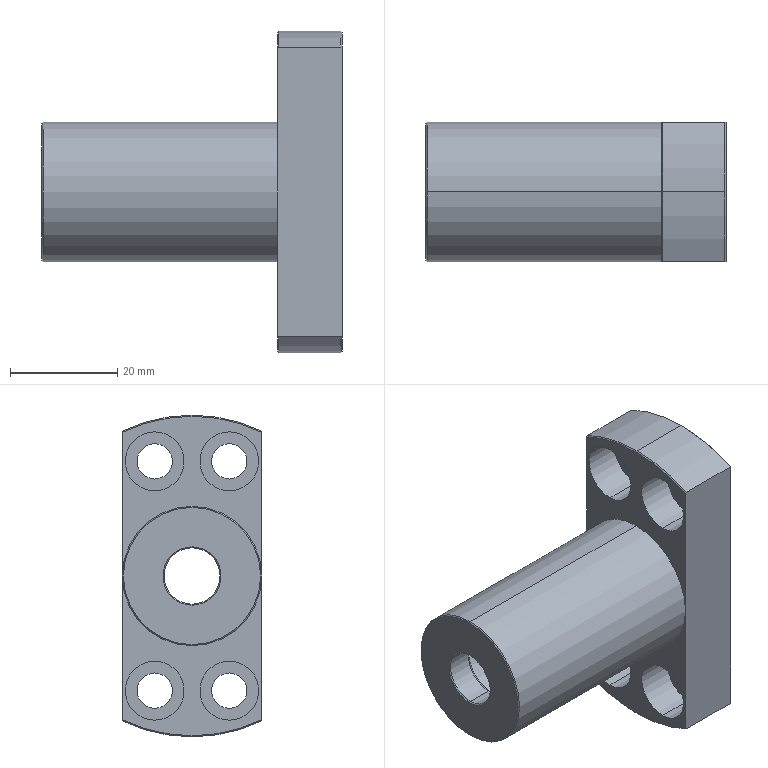Part | SolidWorks | features Chamfer 3, ICE 2, 3DProfileFeature 1, HoleWzd 1, Revolution 1 | 1 solid | 50 faces | box 56 x 26 x 60 mm | volume 18631 mm3 | cylinder 25 | cone 14 | plane 11 | commonest cylinder face diameters 6.6 x8 11 x8 60 x3 10.5 x2 22 x2 26 x2
STEP:
#1=CARTESIAN_POINT('',(5.,0.,5.25));
#2=VERTEX_POINT('',#1);
#3=CARTESIAN_POINT('',(5.,0.,-5.25));
#4=VERTEX_POINT('',#3);
#5=CARTESIAN_POINT('',(5.,0.,0.));
#6=DIRECTION('',(1.,0.,0.));
#7=DIRECTION('',(0.,0.,1.));
#8=AXIS2_PLACEMENT_3D('',#5,#6,#7);
#9=CIRCLE('',#8,5.25);
#10=EDGE_CURVE('',#2,#4,#9,.T.);
#11=ORIENTED_EDGE('',*,*,#10,.F.);
#12=CARTESIAN_POINT('',(6.,0.,6.25));
#13=VERTEX_POINT('',#12);
#14=CARTESIAN_POINT('',(6.,0.,6.25));
#15=DIRECTION('',(0.7071,0.,0.7071));
#16=VECTOR('',#15,1000.);
#17=LINE('',#14,#16);
#18=EDGE_CURVE('',#2,#13,#17,.T.);
#19=ORIENTED_EDGE('',*,*,#18,.T.);
#20=CARTESIAN_POINT('',(6.,0.,-6.25));
#21=VERTEX_POINT('',#20);
#22=CARTESIAN_POINT('',(6.,0.,0.));
#23=DIRECTION('',(-1.,0.,0.));
#24=DIRECTION('',(0.,0.,1.));
#25=AXIS2_PLACEMENT_3D('',#22,#23,#24);
#26=CIRCLE('',#25,6.25);
#27=EDGE_CURVE('',#21,#13,#26,.T.);
#28=ORIENTED_EDGE('',*,*,#27,.F.);
#29=CARTESIAN_POINT('',(6.,0.,-6.25));
#30=DIRECTION('',(0.7071,0.,-0.7071));
#31=VECTOR('',#30,1000.);
#32=LINE('',#29,#31);
#33=EDGE_CURVE('',#4,#21,#32,.T.);
#34=ORIENTED_EDGE('',*,*,#33,.F.);
#35=EDGE_LOOP('',(#11,#19,#28,#34));
#36=FACE_OUTER_BOUND('',#35,.T.);
#37=CARTESIAN_POINT('',(6.,0.,0.));
#38=DIRECTION('',(1.,0.,0.));
#39=DIRECTION('',(0.,0.,-1.));
#40=AXIS2_PLACEMENT_3D('',#37,#38,#39);
#41=CONICAL_SURFACE('',#40,6.25,0.7854);
#42=ADVANCED_FACE('',(#36),#41,.F.);
#43=CARTESIAN_POINT('',(55.8,0.,11.));
#44=VERTEX_POINT('',#43);
#45=CARTESIAN_POINT('',(55.8,0.,-11.));
#46=VERTEX_POINT('',#45);
#47=CARTESIAN_POINT('',(55.8,0.,0.));
#48=DIRECTION('',(1.,0.,0.));
#49=DIRECTION('',(0.,0.,1.));
#50=AXIS2_PLACEMENT_3D('',#47,#48,#49);
#51=CIRCLE('',#50,11.);
#52=EDGE_CURVE('',#44,#46,#51,.T.);
#53=ORIENTED_EDGE('',*,*,#52,.F.);
#54=CARTESIAN_POINT('',(56.,0.,11.2));
#55=VERTEX_POINT('',#54);
#56=CARTESIAN_POINT('',(56.,0.,11.2));
#57=DIRECTION('',(0.7071,0.,0.7071));
#58=VECTOR('',#57,1000.);
#59=LINE('',#56,#58);
#60=EDGE_CURVE('',#44,#55,#59,.T.);
#61=ORIENTED_EDGE('',*,*,#60,.T.);
#62=CARTESIAN_POINT('',(56.,0.,-11.2));
#63=VERTEX_POINT('',#62);
#64=CARTESIAN_POINT('',(56.,0.,0.));
#65=DIRECTION('',(-1.,0.,0.));
#66=DIRECTION('',(0.,0.,1.));
#67=AXIS2_PLACEMENT_3D('',#64,#65,#66);
#68=CIRCLE('',#67,11.2);
#69=EDGE_CURVE('',#63,#55,#68,.T.);
#70=ORIENTED_EDGE('',*,*,#69,.F.);
#71=CARTESIAN_POINT('',(56.,0.,-11.2));
#72=DIRECTION('',(0.7071,0.,-0.7071));
#73=VECTOR('',#72,1000.);
#74=LINE('',#71,#73);
#75=EDGE_CURVE('',#46,#63,#74,.T.);
#76=ORIENTED_EDGE('',*,*,#75,.F.);
#77=EDGE_LOOP('',(#53,#61,#70,#76));
#78=FACE_OUTER_BOUND('',#77,.T.);
#79=CARTESIAN_POINT('',(56.,0.,0.));
#80=DIRECTION('',(1.,0.,0.));
#81=DIRECTION('',(0.,0.,-1.));
#82=AXIS2_PLACEMENT_3D('',#79,#80,#81);
#83=CONICAL_SURFACE('',#82,11.2,0.7854);
#84=ADVANCED_FACE('',(#78),#83,.F.);
#85=CARTESIAN_POINT('',(0.,0.,12.8));
#86=VERTEX_POINT('',#85);
#87=CARTESIAN_POINT('',(0.,0.,-12.8));
#88=VERTEX_POINT('',#87);
#89=CARTESIAN_POINT('',(0.,0.,0.));
#90=DIRECTION('',(-1.,0.,0.));
#91=DIRECTION('',(0.,0.,-1.));
#92=AXIS2_PLACEMENT_3D('',#89,#90,#91);
#93=CIRCLE('',#92,12.8);
#94=EDGE_CURVE('',#86,#88,#93,.T.);
#95=ORIENTED_EDGE('',*,*,#94,.F.);
#96=CARTESIAN_POINT('',(0.2,0.,13.));
#97=VERTEX_POINT('',#96);
#98=CARTESIAN_POINT('',(0.,0.,12.8));
#99=DIRECTION('',(0.7071,0.,0.7071));
#100=VECTOR('',#99,1000.);
#101=LINE('',#98,#100);
#102=EDGE_CURVE('',#86,#97,#101,.T.);
#103=ORIENTED_EDGE('',*,*,#102,.T.);
#104=CARTESIAN_POINT('',(0.2,0.,-13.));
#105=VERTEX_POINT('',#104);
#106=CARTESIAN_POINT('',(0.2,0.,0.));
#107=DIRECTION('',(1.,0.,0.));
#108=DIRECTION('',(0.,0.,-1.));
#109=AXIS2_PLACEMENT_3D('',#106,#107,#108);
#110=CIRCLE('',#109,13.);
#111=EDGE_CURVE('',#105,#97,#110,.T.);
#112=ORIENTED_EDGE('',*,*,#111,.F.);
#113=CARTESIAN_POINT('',(0.,0.,-12.8));
#114=DIRECTION('',(0.7071,0.,-0.7071));
#115=VECTOR('',#114,1000.);
#116=LINE('',#113,#115);
#117=EDGE_CURVE('',#88,#105,#116,.T.);
#118=ORIENTED_EDGE('',*,*,#117,.F.);
#119=EDGE_LOOP('',(#95,#103,#112,#118));
#120=FACE_OUTER_BOUND('',#119,.T.);
#121=CARTESIAN_POINT('',(0.,0.,0.));
#122=DIRECTION('',(1.,0.,0.));
#123=DIRECTION('',(0.,0.,-1.));
#124=AXIS2_PLACEMENT_3D('',#121,#122,#123);
#125=CONICAL_SURFACE('',#124,12.8,0.7854);
#126=ADVANCED_FACE('',(#120),#125,.T.);
#127=CARTESIAN_POINT('',(0.2,0.,-5.25));
#128=VERTEX_POINT('',#127);
#129=CARTESIAN_POINT('',(0.2,0.,5.25));
#130=VERTEX_POINT('',#129);
#131=CARTESIAN_POINT('',(0.2,0.,0.));
#132=DIRECTION('',(-1.,0.,0.));
#133=DIRECTION('',(0.,0.,-1.));
#134=AXIS2_PLACEMENT_3D('',#131,#132,#133);
#135=CIRCLE('',#134,5.25);
#136=EDGE_CURVE('',#128,#130,#135,.T.);
#137=ORIENTED_EDGE('',*,*,#136,.F.);
#138=CARTESIAN_POINT('',(0.,0.,-5.45));
#139=VERTEX_POINT('',#138);
#140=CARTESIAN_POINT('',(0.2,0.,-5.25));
#141=DIRECTION('',(-0.7071,0.,-0.7071));
#142=VECTOR('',#141,1000.);
#143=LINE('',#140,#142);
#144=EDGE_CURVE('',#128,#139,#143,.T.);
#145=ORIENTED_EDGE('',*,*,#144,.T.);
#146=CARTESIAN_POINT('',(0.,0.,5.45));
#147=VERTEX_POINT('',#146);
#148=CARTESIAN_POINT('',(0.,0.,0.));
#149=DIRECTION('',(1.,0.,0.));
#150=DIRECTION('',(0.,0.,-1.));
#151=AXIS2_PLACEMENT_3D('',#148,#149,#150);
#152=CIRCLE('',#151,5.45);
#153=EDGE_CURVE('',#147,#139,#152,.T.);
#154=ORIENTED_EDGE('',*,*,#153,.F.);
#155=CARTESIAN_POINT('',(0.2,0.,5.25));
#156=DIRECTION('',(-0.7071,0.,0.7071));
#157=VECTOR('',#156,1000.);
#158=LINE('',#155,#157);
#159=EDGE_CURVE('',#130,#147,#158,.T.);
#160=ORIENTED_EDGE('',*,*,#159,.F.);
#161=EDGE_LOOP('',(#137,#145,#154,#160));
#162=FACE_OUTER_BOUND('',#161,.T.);
#163=CARTESIAN_POINT('',(0.2,0.,0.));
#164=DIRECTION('',(-1.,0.,0.));
#165=DIRECTION('',(0.,0.,1.));
#166=AXIS2_PLACEMENT_3D('',#163,#164,#165);
#167=CONICAL_SURFACE('',#166,5.25,0.7854);
#168=ADVANCED_FACE('',(#162),#167,.F.);
#169=CARTESIAN_POINT('',(56.,0.,29.8));
#170=VERTEX_POINT('',#169);
#171=CARTESIAN_POINT('',(56.,-13.,26.815));
#172=VERTEX_POINT('',#171);
#173=CARTESIAN_POINT('',(56.,0.,0.));
#174=DIRECTION('',(1.,0.,0.));
#175=DIRECTION('',(0.,0.,1.));
#176=AXIS2_PLACEMENT_3D('',#173,#174,#175);
#177=CIRCLE('',#176,29.8);
#178=EDGE_CURVE('',#170,#172,#177,.T.);
#179=ORIENTED_EDGE('',*,*,#178,.F.);
#180=CARTESIAN_POINT('',(55.8,0.,30.));
#181=VERTEX_POINT('',#180);
#182=CARTESIAN_POINT('',(55.8,0.,30.));
#183=DIRECTION('',(-0.7071,0.,0.7071));
#184=VECTOR('',#183,1000.);
#185=LINE('',#182,#184);
#186=EDGE_CURVE('',#170,#181,#185,.T.);
#187=ORIENTED_EDGE('',*,*,#186,.T.);
#188=CARTESIAN_POINT('',(55.8,-13.,27.037));
#189=VERTEX_POINT('',#188);
#190=CARTESIAN_POINT('',(55.8,0.,0.));
#191=DIRECTION('',(-1.,0.,0.));
#192=DIRECTION('',(0.,0.,1.));
#193=AXIS2_PLACEMENT_3D('',#190,#191,#192);
#194=CIRCLE('',#193,30.);
#195=EDGE_CURVE('',#189,#181,#194,.T.);
#196=ORIENTED_EDGE('',*,*,#195,.F.);
#197=CARTESIAN_POINT('',(56.,-13.,26.815));
#198=CARTESIAN_POINT('',(55.933,-13.,26.889));
#199=CARTESIAN_POINT('',(55.867,-13.,26.963));
#200=CARTESIAN_POINT('',(55.8,-13.,27.037));
#201=B_SPLINE_CURVE_WITH_KNOTS('',3,(#197,#198,#199,#200),.UNSPECIFIED.,.F.,.F.,(4,4),(0.,0.0002989),.UNSPECIFIED.);
#202=EDGE_CURVE('',#172,#189,#201,.T.);
#203=ORIENTED_EDGE('',*,*,#202,.F.);
#204=EDGE_LOOP('',(#179,#187,#196,#203));
#205=FACE_OUTER_BOUND('',#204,.T.);
#206=CARTESIAN_POINT('',(55.8,0.,0.));
#207=DIRECTION('',(-1.,0.,0.));
#208=DIRECTION('',(0.,0.,1.));
#209=AXIS2_PLACEMENT_3D('',#206,#207,#208);
#210=CONICAL_SURFACE('',#209,30.,0.7854);
#211=ADVANCED_FACE('',(#205),#210,.T.);
#212=CARTESIAN_POINT('',(44.,0.,-29.8));
#213=VERTEX_POINT('',#212);
#214=CARTESIAN_POINT('',(44.,-13.,-26.815));
#215=VERTEX_POINT('',#214);
#216=CARTESIAN_POINT('',(44.,0.,0.));
#217=DIRECTION('',(-1.,0.,0.));
#218=DIRECTION('',(0.,0.,-1.));
#219=AXIS2_PLACEMENT_3D('',#216,#217,#218);
#220=CIRCLE('',#219,29.8);
#221=EDGE_CURVE('',#213,#215,#220,.T.);
#222=ORIENTED_EDGE('',*,*,#221,.F.);
#223=CARTESIAN_POINT('',(44.2,0.,-30.));
#224=VERTEX_POINT('',#223);
#225=CARTESIAN_POINT('',(44.,0.,-29.8));
#226=DIRECTION('',(0.7071,0.,-0.7071));
#227=VECTOR('',#226,1000.);
#228=LINE('',#225,#227);
#229=EDGE_CURVE('',#213,#224,#228,.T.);
#230=ORIENTED_EDGE('',*,*,#229,.T.);
#231=CARTESIAN_POINT('',(44.2,-13.,-27.037));
#232=VERTEX_POINT('',#231);
#233=CARTESIAN_POINT('',(44.2,0.,0.));
#234=DIRECTION('',(1.,0.,0.));
#235=DIRECTION('',(0.,0.,-1.));
#236=AXIS2_PLACEMENT_3D('',#233,#234,#235);
#237=CIRCLE('',#236,30.);
#238=EDGE_CURVE('',#232,#224,#237,.T.);
#239=ORIENTED_EDGE('',*,*,#238,.F.);
#240=CARTESIAN_POINT('',(44.,-13.,-26.815));
#241=CARTESIAN_POINT('',(44.067,-13.,-26.889));
#242=CARTESIAN_POINT('',(44.133,-13.,-26.963));
#243=CARTESIAN_POINT('',(44.2,-13.,-27.037));
#244=B_SPLINE_CURVE_WITH_KNOTS('',3,(#240,#241,#242,#243),.UNSPECIFIED.,.F.,.F.,(4,4),(0.,0.0002989),.UNSPECIFIED.);
#245=EDGE_CURVE('',#215,#232,#244,.T.);
#246=ORIENTED_EDGE('',*,*,#245,.F.);
#247=EDGE_LOOP('',(#222,#230,#239,#246));
#248=FACE_OUTER_BOUND('',#247,.T.);
#249=CARTESIAN_POINT('',(44.,0.,0.));
#250=DIRECTION('',(1.,0.,0.));
#251=DIRECTION('',(0.,0.,-1.));
#252=AXIS2_PLACEMENT_3D('',#249,#250,#251);
#253=CONICAL_SURFACE('',#252,29.8,0.7854);
#254=ADVANCED_FACE('',(#248),#253,.T.);
#255=CARTESIAN_POINT('',(50.8,-6.953,15.899));
#256=VERTEX_POINT('',#255);
#257=CARTESIAN_POINT('',(50.8,-6.953,26.899));
#258=VERTEX_POINT('',#257);
#259=CARTESIAN_POINT('',(50.8,-6.953,21.399));
#260=DIRECTION('',(-1.,0.,0.));
#261=DIRECTION('',(0.,0.,1.));
#262=AXIS2_PLACEMENT_3D('',#259,#260,#261);
#263=CIRCLE('',#262,5.5);
#264=EDGE_CURVE('',#256,#258,#263,.T.);
#265=ORIENTED_EDGE('',*,*,#264,.F.);
#266=CARTESIAN_POINT('',(44.,-6.953,15.899));
#267=VERTEX_POINT('',#266);
#268=CARTESIAN_POINT('',(44.,-6.953,15.899));
#269=DIRECTION('',(-1.,0.,0.));
#270=VECTOR('',#269,1000.);
#271=LINE('',#268,#270);
#272=EDGE_CURVE('',#256,#267,#271,.T.);
#273=ORIENTED_EDGE('',*,*,#272,.T.);
#274=CARTESIAN_POINT('',(44.,-6.953,26.899));
#275=VERTEX_POINT('',#274);
#276=CARTESIAN_POINT('',(44.,-6.953,21.399));
#277=DIRECTION('',(-1.,0.,0.));
#278=DIRECTION('',(0.,0.,1.));
#279=AXIS2_PLACEMENT_3D('',#276,#277,#278);
#280=CIRCLE('',#279,5.5);
#281=EDGE_CURVE('',#267,#275,#280,.T.);
#282=ORIENTED_EDGE('',*,*,#281,.T.);
#283=CARTESIAN_POINT('',(44.,-6.953,26.899));
#284=DIRECTION('',(-1.,0.,0.));
#285=VECTOR('',#284,1000.);
#286=LINE('',#283,#285);
#287=EDGE_CURVE('',#258,#275,#286,.T.);
#288=ORIENTED_EDGE('',*,*,#287,.F.);
#289=EDGE_LOOP('',(#265,#273,#282,#288));
#290=FACE_OUTER_BOUND('',#289,.T.);
#291=CARTESIAN_POINT('',(44.,-6.953,21.399));
#292=DIRECTION('',(-1.,0.,0.));
#293=DIRECTION('',(0.,0.,1.));
#294=AXIS2_PLACEMENT_3D('',#291,#292,#293);
#295=CYLINDRICAL_SURFACE('',#294,5.5);
#296=ADVANCED_FACE('',(#290),#295,.F.);
#297=CARTESIAN_POINT('',(56.,-6.953,18.099));
#298=VERTEX_POINT('',#297);
#299=CARTESIAN_POINT('',(56.,-6.953,24.699));
#300=VERTEX_POINT('',#299);
#301=CARTESIAN_POINT('',(56.,-6.953,21.399));
#302=DIRECTION('',(-1.,0.,0.));
#303=DIRECTION('',(0.,0.,1.));
#304=AXIS2_PLACEMENT_3D('',#301,#302,#303);
#305=CIRCLE('',#304,3.3);
#306=EDGE_CURVE('',#298,#300,#305,.T.);
#307=ORIENTED_EDGE('',*,*,#306,.F.);
#308=CARTESIAN_POINT('',(50.8,-6.953,18.099));
#309=VERTEX_POINT('',#308);
#310=CARTESIAN_POINT('',(44.,-6.953,18.099));
#311=DIRECTION('',(-1.,0.,0.));
#312=VECTOR('',#311,1000.);
#313=LINE('',#310,#312);
#314=EDGE_CURVE('',#298,#309,#313,.T.);
#315=ORIENTED_EDGE('',*,*,#314,.T.);
#316=CARTESIAN_POINT('',(50.8,-6.953,24.699));
#317=VERTEX_POINT('',#316);
#318=CARTESIAN_POINT('',(50.8,-6.953,21.399));
#319=DIRECTION('',(-1.,0.,0.));
#320=DIRECTION('',(0.,0.,1.));
#321=AXIS2_PLACEMENT_3D('',#318,#319,#320);
#322=CIRCLE('',#321,3.3);
#323=EDGE_CURVE('',#309,#317,#322,.T.);
#324=ORIENTED_EDGE('',*,*,#323,.T.);
#325=CARTESIAN_POINT('',(44.,-6.953,24.699));
#326=DIRECTION('',(-1.,0.,0.));
#327=VECTOR('',#326,1000.);
#328=LINE('',#325,#327);
#329=EDGE_CURVE('',#300,#317,#328,.T.);
#330=ORIENTED_EDGE('',*,*,#329,.F.);
#331=EDGE_LOOP('',(#307,#315,#324,#330));
#332=FACE_OUTER_BOUND('',#331,.T.);
#333=CARTESIAN_POINT('',(44.,-6.953,21.399));
#334=DIRECTION('',(-1.,0.,0.));
#335=DIRECTION('',(0.,0.,1.));
#336=AXIS2_PLACEMENT_3D('',#333,#334,#335);
#337=CYLINDRICAL_SURFACE('',#336,3.3);
#338=ADVANCED_FACE('',(#332),#337,.F.);
#339=CARTESIAN_POINT('',(50.8,6.953,15.899));
#340=VERTEX_POINT('',#339);
#341=CARTESIAN_POINT('',(50.8,6.953,26.899));
#342=VERTEX_POINT('',#341);
#343=CARTESIAN_POINT('',(50.8,6.953,21.399));
#344=DIRECTION('',(-1.,0.,0.));
#345=DIRECTION('',(0.,0.,1.));
#346=AXIS2_PLACEMENT_3D('',#343,#344,#345);
#347=CIRCLE('',#346,5.5);
#348=EDGE_CURVE('',#340,#342,#347,.T.);
#349=ORIENTED_EDGE('',*,*,#348,.F.);
#350=CARTESIAN_POINT('',(44.,6.953,15.899));
#351=VERTEX_POINT('',#350);
#352=CARTESIAN_POINT('',(44.,6.953,15.899));
#353=DIRECTION('',(-1.,0.,0.));
#354=VECTOR('',#353,1000.);
#355=LINE('',#352,#354);
#356=EDGE_CURVE('',#340,#351,#355,.T.);
#357=ORIENTED_EDGE('',*,*,#356,.T.);
#358=CARTESIAN_POINT('',(44.,6.953,26.899));
#359=VERTEX_POINT('',#358);
#360=CARTESIAN_POINT('',(44.,6.953,21.399));
#361=DIRECTION('',(-1.,0.,0.));
#362=DIRECTION('',(0.,0.,1.));
#363=AXIS2_PLACEMENT_3D('',#360,#361,#362);
#364=CIRCLE('',#363,5.5);
#365=EDGE_CURVE('',#351,#359,#364,.T.);
#366=ORIENTED_EDGE('',*,*,#365,.T.);
#367=CARTESIAN_POINT('',(44.,6.953,26.899));
#368=DIRECTION('',(-1.,0.,0.));
#369=VECTOR('',#368,1000.);
#370=LINE('',#367,#369);
#371=EDGE_CURVE('',#342,#359,#370,.T.);
#372=ORIENTED_EDGE('',*,*,#371,.F.);
#373=EDGE_LOOP('',(#349,#357,#366,#372));
#374=FACE_OUTER_BOUND('',#373,.T.);
#375=CARTESIAN_POINT('',(44.,6.953,21.399));
#376=DIRECTION('',(-1.,0.,0.));
#377=DIRECTION('',(0.,0.,1.));
#378=AXIS2_PLACEMENT_3D('',#375,#376,#377);
#379=CYLINDRICAL_SURFACE('',#378,5.5);
#380=ADVANCED_FACE('',(#374),#379,.F.);
#381=CARTESIAN_POINT('',(56.,6.953,18.099));
#382=VERTEX_POINT('',#381);
#383=CARTESIAN_POINT('',(56.,6.953,24.699));
#384=VERTEX_POINT('',#383);
#385=CARTESIAN_POINT('',(56.,6.953,21.399));
#386=DIRECTION('',(-1.,0.,0.));
#387=DIRECTION('',(0.,0.,1.));
#388=AXIS2_PLACEMENT_3D('',#385,#386,#387);
#389=CIRCLE('',#388,3.3);
#390=EDGE_CURVE('',#382,#384,#389,.T.);
#391=ORIENTED_EDGE('',*,*,#390,.F.);
#392=CARTESIAN_POINT('',(50.8,6.953,18.099));
#393=VERTEX_POINT('',#392);
#394=CARTESIAN_POINT('',(44.,6.953,18.099));
#395=DIRECTION('',(-1.,0.,0.));
#396=VECTOR('',#395,1000.);
#397=LINE('',#394,#396);
#398=EDGE_CURVE('',#382,#393,#397,.T.);
#399=ORIENTED_EDGE('',*,*,#398,.T.);
#400=CARTESIAN_POINT('',(50.8,6.953,24.699));
#401=VERTEX_POINT('',#400);
#402=CARTESIAN_POINT('',(50.8,6.953,21.399));
#403=DIRECTION('',(-1.,0.,0.));
#404=DIRECTION('',(0.,0.,1.));
#405=AXIS2_PLACEMENT_3D('',#402,#403,#404);
#406=CIRCLE('',#405,3.3);
#407=EDGE_CURVE('',#393,#401,#406,.T.);
#408=ORIENTED_EDGE('',*,*,#407,.T.);
#409=CARTESIAN_POINT('',(44.,6.953,24.699));
#410=DIRECTION('',(-1.,0.,0.));
#411=VECTOR('',#410,1000.);
#412=LINE('',#409,#411);
#413=EDGE_CURVE('',#384,#401,#412,.T.);
#414=ORIENTED_EDGE('',*,*,#413,.F.);
#415=EDGE_LOOP('',(#391,#399,#408,#414));
#416=FACE_OUTER_BOUND('',#415,.T.);
#417=CARTESIAN_POINT('',(44.,6.953,21.399));
#418=DIRECTION('',(-1.,0.,0.));
#419=DIRECTION('',(0.,0.,1.));
#420=AXIS2_PLACEMENT_3D('',#417,#418,#419);
#421=CYLINDRICAL_SURFACE('',#420,3.3);
#422=ADVANCED_FACE('',(#416),#421,.F.);
#423=CARTESIAN_POINT('',(50.8,6.953,-26.899));
#424=VERTEX_POINT('',#423);
#425=CARTESIAN_POINT('',(50.8,6.953,-15.899));
#426=VERTEX_POINT('',#425);
#427=CARTESIAN_POINT('',(50.8,6.953,-21.399));
#428=DIRECTION('',(-1.,0.,0.));
#429=DIRECTION('',(0.,0.,1.));
#430=AXIS2_PLACEMENT_3D('',#427,#428,#429);
#431=CIRCLE('',#430,5.5);
#432=EDGE_CURVE('',#424,#426,#431,.T.);
#433=ORIENTED_EDGE('',*,*,#432,.F.);
#434=CARTESIAN_POINT('',(44.,6.953,-26.899));
#435=VERTEX_POINT('',#434);
#436=CARTESIAN_POINT('',(44.,6.953,-26.899));
#437=DIRECTION('',(-1.,0.,0.));
#438=VECTOR('',#437,1000.);
#439=LINE('',#436,#438);
#440=EDGE_CURVE('',#424,#435,#439,.T.);
#441=ORIENTED_EDGE('',*,*,#440,.T.);
#442=CARTESIAN_POINT('',(44.,6.953,-15.899));
#443=VERTEX_POINT('',#442);
#444=CARTESIAN_POINT('',(44.,6.953,-21.399));
#445=DIRECTION('',(-1.,0.,0.));
#446=DIRECTION('',(0.,0.,1.));
#447=AXIS2_PLACEMENT_3D('',#444,#445,#446);
#448=CIRCLE('',#447,5.5);
#449=EDGE_CURVE('',#435,#443,#448,.T.);
#450=ORIENTED_EDGE('',*,*,#449,.T.);
#451=CARTESIAN_POINT('',(44.,6.953,-15.899));
#452=DIRECTION('',(-1.,0.,0.));
#453=VECTOR('',#452,1000.);
#454=LINE('',#451,#453);
#455=EDGE_CURVE('',#426,#443,#454,.T.);
#456=ORIENTED_EDGE('',*,*,#455,.F.);
#457=EDGE_LOOP('',(#433,#441,#450,#456));
#458=FACE_OUTER_BOUND('',#457,.T.);
#459=CARTESIAN_POINT('',(44.,6.953,-21.399));
#460=DIRECTION('',(-1.,0.,0.));
#461=DIRECTION('',(0.,0.,1.));
#462=AXIS2_PLACEMENT_3D('',#459,#460,#461);
#463=CYLINDRICAL_SURFACE('',#462,5.5);
#464=ADVANCED_FACE('',(#458),#463,.F.);
#465=CARTESIAN_POINT('',(56.,6.953,-24.699));
#466=VERTEX_POINT('',#465);
#467=CARTESIAN_POINT('',(56.,6.953,-18.099));
#468=VERTEX_POINT('',#467);
#469=CARTESIAN_POINT('',(56.,6.953,-21.399));
#470=DIRECTION('',(-1.,0.,0.));
#471=DIRECTION('',(0.,0.,1.));
#472=AXIS2_PLACEMENT_3D('',#469,#470,#471);
#473=CIRCLE('',#472,3.3);
#474=EDGE_CURVE('',#466,#468,#473,.T.);
#475=ORIENTED_EDGE('',*,*,#474,.F.);
#476=CARTESIAN_POINT('',(50.8,6.953,-24.699));
#477=VERTEX_POINT('',#476);
#478=CARTESIAN_POINT('',(44.,6.953,-24.699));
#479=DIRECTION('',(-1.,0.,0.));
#480=VECTOR('',#479,1000.);
#481=LINE('',#478,#480);
#482=EDGE_CURVE('',#466,#477,#481,.T.);
#483=ORIENTED_EDGE('',*,*,#482,.T.);
#484=CARTESIAN_POINT('',(50.8,6.953,-18.099));
#485=VERTEX_POINT('',#484);
#486=CARTESIAN_POINT('',(50.8,6.953,-21.399));
#487=DIRECTION('',(-1.,0.,0.));
#488=DIRECTION('',(0.,0.,1.));
#489=AXIS2_PLACEMENT_3D('',#486,#487,#488);
#490=CIRCLE('',#489,3.3);
#491=EDGE_CURVE('',#477,#485,#490,.T.);
#492=ORIENTED_EDGE('',*,*,#491,.T.);
#493=CARTESIAN_POINT('',(44.,6.953,-18.099));
#494=DIRECTION('',(-1.,0.,0.));
#495=VECTOR('',#494,1000.);
#496=LINE('',#493,#495);
#497=EDGE_CURVE('',#468,#485,#496,.T.);
#498=ORIENTED_EDGE('',*,*,#497,.F.);
#499=EDGE_LOOP('',(#475,#483,#492,#498));
#500=FACE_OUTER_BOUND('',#499,.T.);
#501=CARTESIAN_POINT('',(44.,6.953,-21.399));
#502=DIRECTION('',(-1.,0.,0.));
#503=DIRECTION('',(0.,0.,1.));
#504=AXIS2_PLACEMENT_3D('',#501,#502,#503);
#505=CYLINDRICAL_SURFACE('',#504,3.3);
#506=ADVANCED_FACE('',(#500),#505,.F.);
#507=CARTESIAN_POINT('',(50.8,-6.953,-26.899));
#508=VERTEX_POINT('',#507);
#509=CARTESIAN_POINT('',(50.8,-6.953,-15.899));
#510=VERTEX_POINT('',#509);
#511=CARTESIAN_POINT('',(50.8,-6.953,-21.399));
#512=DIRECTION('',(-1.,0.,0.));
#513=DIRECTION('',(0.,0.,1.));
#514=AXIS2_PLACEMENT_3D('',#511,#512,#513);
#515=CIRCLE('',#514,5.5);
#516=EDGE_CURVE('',#508,#510,#515,.T.);
#517=ORIENTED_EDGE('',*,*,#516,.F.);
#518=CARTESIAN_POINT('',(44.,-6.953,-26.899));
#519=VERTEX_POINT('',#518);
#520=CARTESIAN_POINT('',(44.,-6.953,-26.899));
#521=DIRECTION('',(-1.,0.,0.));
#522=VECTOR('',#521,1000.);
#523=LINE('',#520,#522);
#524=EDGE_CURVE('',#508,#519,#523,.T.);
#525=ORIENTED_EDGE('',*,*,#524,.T.);
#526=CARTESIAN_POINT('',(44.,-6.953,-15.899));
#527=VERTEX_POINT('',#526);
#528=CARTESIAN_POINT('',(44.,-6.953,-21.399));
#529=DIRECTION('',(-1.,0.,0.));
#530=DIRECTION('',(0.,0.,1.));
#531=AXIS2_PLACEMENT_3D('',#528,#529,#530);
#532=CIRCLE('',#531,5.5);
#533=EDGE_CURVE('',#519,#527,#532,.T.);
#534=ORIENTED_EDGE('',*,*,#533,.T.);
#535=CARTESIAN_POINT('',(44.,-6.953,-15.899));
#536=DIRECTION('',(-1.,0.,0.));
#537=VECTOR('',#536,1000.);
#538=LINE('',#535,#537);
#539=EDGE_CURVE('',#510,#527,#538,.T.);
#540=ORIENTED_EDGE('',*,*,#539,.F.);
#541=EDGE_LOOP('',(#517,#525,#534,#540));
#542=FACE_OUTER_BOUND('',#541,.T.);
#543=CARTESIAN_POINT('',(44.,-6.953,-21.399));
#544=DIRECTION('',(-1.,0.,0.));
#545=DIRECTION('',(0.,0.,1.));
#546=AXIS2_PLACEMENT_3D('',#543,#544,#545);
#547=CYLINDRICAL_SURFACE('',#546,5.5);
#548=ADVANCED_FACE('',(#542),#547,.F.);
#549=CARTESIAN_POINT('',(56.,-6.953,-24.699));
#550=VERTEX_POINT('',#549);
#551=CARTESIAN_POINT('',(56.,-6.953,-18.099));
#552=VERTEX_POINT('',#551);
#553=CARTESIAN_POINT('',(56.,-6.953,-21.399));
#554=DIRECTION('',(-1.,0.,0.));
#555=DIRECTION('',(0.,0.,1.));
#556=AXIS2_PLACEMENT_3D('',#553,#554,#555);
#557=CIRCLE('',#556,3.3);
#558=EDGE_CURVE('',#550,#552,#557,.T.);
#559=ORIENTED_EDGE('',*,*,#558,.F.);
#560=CARTESIAN_POINT('',(50.8,-6.953,-24.699));
#561=VERTEX_POINT('',#560);
#562=CARTESIAN_POINT('',(44.,-6.953,-24.699));
#563=DIRECTION('',(-1.,0.,0.));
#564=VECTOR('',#563,1000.);
#565=LINE('',#562,#564);
#566=EDGE_CURVE('',#550,#561,#565,.T.);
#567=ORIENTED_EDGE('',*,*,#566,.T.);
#568=CARTESIAN_POINT('',(50.8,-6.953,-18.099));
#569=VERTEX_POINT('',#568);
#570=CARTESIAN_POINT('',(50.8,-6.953,-21.399));
#571=DIRECTION('',(-1.,0.,0.));
#572=DIRECTION('',(0.,0.,1.));
#573=AXIS2_PLACEMENT_3D('',#570,#571,#572);
#574=CIRCLE('',#573,3.3);
#575=EDGE_CURVE('',#561,#569,#574,.T.);
#576=ORIENTED_EDGE('',*,*,#575,.T.);
#577=CARTESIAN_POINT('',(44.,-6.953,-18.099));
#578=DIRECTION('',(-1.,0.,0.));
#579=VECTOR('',#578,1000.);
#580=LINE('',#577,#579);
#581=EDGE_CURVE('',#552,#569,#580,.T.);
#582=ORIENTED_EDGE('',*,*,#581,.F.);
#583=EDGE_LOOP('',(#559,#567,#576,#582));
#584=FACE_OUTER_BOUND('',#583,.T.);
#585=CARTESIAN_POINT('',(44.,-6.953,-21.399));
#586=DIRECTION('',(-1.,0.,0.));
#587=DIRECTION('',(0.,0.,1.));
#588=AXIS2_PLACEMENT_3D('',#585,#586,#587);
#589=CYLINDRICAL_SURFACE('',#588,3.3);
#590=ADVANCED_FACE('',(#584),#589,.F.);
#591=ORIENTED_EDGE('',*,*,#10,.T.);
#592=CARTESIAN_POINT('',(56.,0.,-5.25));
#593=DIRECTION('',(-1.,0.,0.));
#594=VECTOR('',#593,1000.);
#595=LINE('',#592,#594);
#596=EDGE_CURVE('',#4,#128,#595,.T.);
#597=ORIENTED_EDGE('',*,*,#596,.T.);
#598=ORIENTED_EDGE('',*,*,#136,.T.);
#599=CARTESIAN_POINT('',(56.,0.,5.25));
#600=DIRECTION('',(-1.,0.,0.));
#601=VECTOR('',#600,1000.);
#602=LINE('',#599,#601);
#603=EDGE_CURVE('',#2,#130,#602,.T.);
#604=ORIENTED_EDGE('',*,*,#603,.F.);
#605=EDGE_LOOP('',(#591,#597,#598,#604));
#606=FACE_OUTER_BOUND('',#605,.T.);
#607=CARTESIAN_POINT('',(56.,0.,0.));
#608=DIRECTION('',(-1.,0.,0.));
#609=DIRECTION('',(0.,0.,1.));
#610=AXIS2_PLACEMENT_3D('',#607,#608,#609);
#611=CYLINDRICAL_SURFACE('',#610,5.25);
#612=ADVANCED_FACE('',(#606),#611,.F.);
#613=ORIENTED_EDGE('',*,*,#52,.T.);
#614=CARTESIAN_POINT('',(6.,0.,-11.));
#615=VERTEX_POINT('',#614);
#616=CARTESIAN_POINT('',(0.,0.,-11.));
#617=DIRECTION('',(-1.,0.,0.));
#618=VECTOR('',#617,1000.);
#619=LINE('',#616,#618);
#620=EDGE_CURVE('',#46,#615,#619,.T.);
#621=ORIENTED_EDGE('',*,*,#620,.T.);
#622=CARTESIAN_POINT('',(6.,0.,11.));
#623=VERTEX_POINT('',#622);
#624=CARTESIAN_POINT('',(6.,0.,0.));
#625=DIRECTION('',(-1.,0.,0.));
#626=DIRECTION('',(0.,0.,1.));
#627=AXIS2_PLACEMENT_3D('',#624,#625,#626);
#628=CIRCLE('',#627,11.);
#629=EDGE_CURVE('',#615,#623,#628,.T.);
#630=ORIENTED_EDGE('',*,*,#629,.T.);
#631=CARTESIAN_POINT('',(0.,0.,11.));
#632=DIRECTION('',(-1.,0.,0.));
#633=VECTOR('',#632,1000.);
#634=LINE('',#631,#633);
#635=EDGE_CURVE('',#44,#623,#634,.T.);
#636=ORIENTED_EDGE('',*,*,#635,.F.);
#637=EDGE_LOOP('',(#613,#621,#630,#636));
#638=FACE_OUTER_BOUND('',#637,.T.);
#639=CARTESIAN_POINT('',(0.,0.,0.));
#640=DIRECTION('',(-1.,0.,0.));
#641=DIRECTION('',(0.,0.,1.));
#642=AXIS2_PLACEMENT_3D('',#639,#640,#641);
#643=CYLINDRICAL_SURFACE('',#642,11.);
#644=ADVANCED_FACE('',(#638),#643,.F.);
#645=CARTESIAN_POINT('',(44.,13.,0.));
#646=VERTEX_POINT('',#645);
#647=CARTESIAN_POINT('',(44.,0.,-13.));
#648=VERTEX_POINT('',#647);
#649=CARTESIAN_POINT('',(44.,0.,0.));
#650=DIRECTION('',(-1.,0.,0.));
#651=DIRECTION('',(0.,0.,1.));
#652=AXIS2_PLACEMENT_3D('',#649,#650,#651);
#653=CIRCLE('',#652,13.);
#654=EDGE_CURVE('',#646,#648,#653,.T.);
#655=ORIENTED_EDGE('',*,*,#654,.T.);
#656=CARTESIAN_POINT('',(0.,0.,-13.));
#657=DIRECTION('',(-1.,0.,0.));
#658=VECTOR('',#657,1000.);
#659=LINE('',#656,#658);
#660=EDGE_CURVE('',#648,#105,#659,.T.);
#661=ORIENTED_EDGE('',*,*,#660,.T.);
#662=ORIENTED_EDGE('',*,*,#111,.T.);
#663=CARTESIAN_POINT('',(44.,0.,13.));
#664=VERTEX_POINT('',#663);
#665=CARTESIAN_POINT('',(0.,0.,13.));
#666=DIRECTION('',(-1.,0.,0.));
#667=VECTOR('',#666,1000.);
#668=LINE('',#665,#667);
#669=EDGE_CURVE('',#664,#97,#668,.T.);
#670=ORIENTED_EDGE('',*,*,#669,.F.);
#671=CARTESIAN_POINT('',(44.,0.,0.));
#672=DIRECTION('',(-1.,0.,0.));
#673=DIRECTION('',(0.,0.,1.));
#674=AXIS2_PLACEMENT_3D('',#671,#672,#673);
#675=CIRCLE('',#674,13.);
#676=EDGE_CURVE('',#664,#646,#675,.T.);
#677=ORIENTED_EDGE('',*,*,#676,.T.);
#678=EDGE_LOOP('',(#655,#661,#662,#670,#677));
#679=FACE_OUTER_BOUND('',#678,.T.);
#680=CARTESIAN_POINT('',(0.,0.,0.));
#681=DIRECTION('',(-1.,0.,0.));
#682=DIRECTION('',(0.,0.,1.));
#683=AXIS2_PLACEMENT_3D('',#680,#681,#682);
#684=CYLINDRICAL_SURFACE('',#683,13.);
#685=ADVANCED_FACE('',(#679),#684,.T.);
#686=ORIENTED_EDGE('',*,*,#195,.T.);
#687=CARTESIAN_POINT('',(44.2,0.,30.));
#688=VERTEX_POINT('',#687);
#689=CARTESIAN_POINT('',(0.,0.,30.));
#690=DIRECTION('',(-1.,0.,0.));
#691=VECTOR('',#690,1000.);
#692=LINE('',#689,#691);
#693=EDGE_CURVE('',#181,#688,#692,.T.);
#694=ORIENTED_EDGE('',*,*,#693,.T.);
#695=CARTESIAN_POINT('',(44.2,-13.,27.037));
#696=VERTEX_POINT('',#695);
#697=CARTESIAN_POINT('',(44.2,0.,0.));
#698=DIRECTION('',(1.,0.,0.));
#699=DIRECTION('',(0.,0.,-1.));
#700=AXIS2_PLACEMENT_3D('',#697,#698,#699);
#701=CIRCLE('',#700,30.);
#702=EDGE_CURVE('',#688,#696,#701,.T.);
#703=ORIENTED_EDGE('',*,*,#702,.T.);
#704=CARTESIAN_POINT('',(56.001,-13.,27.037));
#705=DIRECTION('',(-1.,0.,0.));
#706=VECTOR('',#705,1000.);
#707=LINE('',#704,#706);
#708=EDGE_CURVE('',#189,#696,#707,.T.);
#709=ORIENTED_EDGE('',*,*,#708,.F.);
#710=EDGE_LOOP('',(#686,#694,#703,#709));
#711=FACE_OUTER_BOUND('',#710,.T.);
#712=CARTESIAN_POINT('',(0.,0.,0.));
#713=DIRECTION('',(-1.,0.,0.));
#714=DIRECTION('',(0.,0.,1.));
#715=AXIS2_PLACEMENT_3D('',#712,#713,#714);
#716=CYLINDRICAL_SURFACE('',#715,30.);
#717=ADVANCED_FACE('',(#711),#716,.T.);
#718=CARTESIAN_POINT('',(44.,-6.953,21.399));
#719=DIRECTION('',(-1.,0.,0.));
#720=DIRECTION('',(0.,0.,1.));
#721=AXIS2_PLACEMENT_3D('',#718,#719,#720);
#722=CIRCLE('',#721,5.5);
#723=EDGE_CURVE('',#275,#267,#722,.T.);
#724=ORIENTED_EDGE('',*,*,#723,.F.);
#725=ORIENTED_EDGE('',*,*,#281,.F.);
#726=EDGE_LOOP('',(#724,#725));
#727=FACE_BOUND('',#726,.T.);
#728=CARTESIAN_POINT('',(44.,6.953,21.399));
#729=DIRECTION('',(-1.,0.,0.));
#730=DIRECTION('',(0.,0.,1.));
#731=AXIS2_PLACEMENT_3D('',#728,#729,#730);
#732=CIRCLE('',#731,5.5);
#733=EDGE_CURVE('',#359,#351,#732,.T.);
#734=ORIENTED_EDGE('',*,*,#733,.F.);
#735=ORIENTED_EDGE('',*,*,#365,.F.);
#736=EDGE_LOOP('',(#734,#735));
#737=FACE_BOUND('',#736,.T.);
#738=CARTESIAN_POINT('',(44.,-13.,26.815));
#739=VERTEX_POINT('',#738);
#740=CARTESIAN_POINT('',(44.,-13.,0.));
#741=VERTEX_POINT('',#740);
#742=CARTESIAN_POINT('',(44.,-13.,27.037));
#743=DIRECTION('',(0.,0.,-1.));
#744=VECTOR('',#743,1000.);
#745=LINE('',#742,#744);
#746=EDGE_CURVE('',#739,#741,#745,.T.);
#747=ORIENTED_EDGE('',*,*,#746,.F.);
#748=CARTESIAN_POINT('',(44.,13.,26.815));
#749=VERTEX_POINT('',#748);
#750=CARTESIAN_POINT('',(44.,0.,0.));
#751=DIRECTION('',(-1.,0.,0.));
#752=DIRECTION('',(0.,0.,-1.));
#753=AXIS2_PLACEMENT_3D('',#750,#751,#752);
#754=CIRCLE('',#753,29.8);
#755=EDGE_CURVE('',#739,#749,#754,.T.);
#756=ORIENTED_EDGE('',*,*,#755,.T.);
#757=CARTESIAN_POINT('',(44.,13.,27.037));
#758=DIRECTION('',(0.,0.,1.));
#759=VECTOR('',#758,1000.);
#760=LINE('',#757,#759);
#761=EDGE_CURVE('',#646,#749,#760,.T.);
#762=ORIENTED_EDGE('',*,*,#761,.F.);
#763=ORIENTED_EDGE('',*,*,#676,.F.);
#764=CARTESIAN_POINT('',(44.,0.,0.));
#765=DIRECTION('',(-1.,0.,0.));
#766=DIRECTION('',(0.,0.,1.));
#767=AXIS2_PLACEMENT_3D('',#764,#765,#766);
#768=CIRCLE('',#767,13.);
#769=EDGE_CURVE('',#741,#664,#768,.T.);
#770=ORIENTED_EDGE('',*,*,#769,.F.);
#771=EDGE_LOOP('',(#747,#756,#762,#763,#770));
#772=FACE_OUTER_BOUND('',#771,.T.);
#773=CARTESIAN_POINT('',(44.,13.,0.));
#774=DIRECTION('',(1.,0.,0.));
#775=DIRECTION('',(0.,0.,-1.));
#776=AXIS2_PLACEMENT_3D('',#773,#774,#775);
#777=PLANE('',#776);
#778=ADVANCED_FACE('',(#727,#737,#772),#777,.F.);
#779=ORIENTED_EDGE('',*,*,#693,.F.);
#780=CARTESIAN_POINT('',(55.8,13.,27.037));
#781=VERTEX_POINT('',#780);
#782=CARTESIAN_POINT('',(55.8,0.,0.));
#783=DIRECTION('',(-1.,0.,0.));
#784=DIRECTION('',(0.,0.,1.));
#785=AXIS2_PLACEMENT_3D('',#782,#783,#784);
#786=CIRCLE('',#785,30.);
#787=EDGE_CURVE('',#181,#781,#786,.T.);
#788=ORIENTED_EDGE('',*,*,#787,.T.);
#789=CARTESIAN_POINT('',(44.2,13.,27.037));
#790=VERTEX_POINT('',#789);
#791=CARTESIAN_POINT('',(56.001,13.,27.037));
#792=DIRECTION('',(-1.,0.,0.));
#793=VECTOR('',#792,1000.);
#794=LINE('',#791,#793);
#795=EDGE_CURVE('',#781,#790,#794,.T.);
#796=ORIENTED_EDGE('',*,*,#795,.T.);
#797=CARTESIAN_POINT('',(44.2,0.,0.));
#798=DIRECTION('',(1.,0.,0.));
#799=DIRECTION('',(0.,0.,-1.));
#800=AXIS2_PLACEMENT_3D('',#797,#798,#799);
#801=CIRCLE('',#800,30.);
#802=EDGE_CURVE('',#790,#688,#801,.T.);
#803=ORIENTED_EDGE('',*,*,#802,.T.);
#804=EDGE_LOOP('',(#779,#788,#796,#803));
#805=FACE_OUTER_BOUND('',#804,.T.);
#806=CARTESIAN_POINT('',(0.,0.,0.));
#807=DIRECTION('',(-1.,0.,0.));
#808=DIRECTION('',(0.,0.,1.));
#809=AXIS2_PLACEMENT_3D('',#806,#807,#808);
#810=CYLINDRICAL_SURFACE('',#809,30.);
#811=ADVANCED_FACE('',(#805),#810,.T.);
#812=ORIENTED_EDGE('',*,*,#153,.T.);
#813=CARTESIAN_POINT('',(0.,0.,0.));
#814=DIRECTION('',(1.,0.,0.));
#815=DIRECTION('',(0.,0.,-1.));
#816=AXIS2_PLACEMENT_3D('',#813,#814,#815);
#817=CIRCLE('',#816,5.45);
#818=EDGE_CURVE('',#139,#147,#817,.T.);
#819=ORIENTED_EDGE('',*,*,#818,.T.);
#820=EDGE_LOOP('',(#812,#819));
#821=FACE_BOUND('',#820,.T.);
#822=CARTESIAN_POINT('',(0.,0.,0.));
#823=DIRECTION('',(-1.,0.,0.));
#824=DIRECTION('',(0.,0.,-1.));
#825=AXIS2_PLACEMENT_3D('',#822,#823,#824);
#826=CIRCLE('',#825,12.8);
#827=EDGE_CURVE('',#88,#86,#826,.T.);
#828=ORIENTED_EDGE('',*,*,#827,.T.);
#829=ORIENTED_EDGE('',*,*,#94,.T.);
#830=EDGE_LOOP('',(#828,#829));
#831=FACE_OUTER_BOUND('',#830,.T.);
#832=CARTESIAN_POINT('',(0.,0.,0.));
#833=DIRECTION('',(1.,0.,0.));
#834=DIRECTION('',(0.,0.,-1.));
#835=AXIS2_PLACEMENT_3D('',#832,#833,#834);
#836=PLANE('',#835);
#837=ADVANCED_FACE('',(#821,#831),#836,.F.);
#838=ORIENTED_EDGE('',*,*,#660,.F.);
#839=CARTESIAN_POINT('',(44.,0.,0.));
#840=DIRECTION('',(-1.,0.,0.));
#841=DIRECTION('',(0.,0.,1.));
#842=AXIS2_PLACEMENT_3D('',#839,#840,#841);
#843=CIRCLE('',#842,13.);
#844=EDGE_CURVE('',#648,#741,#843,.T.);
#845=ORIENTED_EDGE('',*,*,#844,.T.);
#846=ORIENTED_EDGE('',*,*,#769,.T.);
#847=ORIENTED_EDGE('',*,*,#669,.T.);
#848=CARTESIAN_POINT('',(0.2,0.,0.));
#849=DIRECTION('',(1.,0.,0.));
#850=DIRECTION('',(0.,0.,-1.));
#851=AXIS2_PLACEMENT_3D('',#848,#849,#850);
#852=CIRCLE('',#851,13.);
#853=EDGE_CURVE('',#97,#105,#852,.T.);
#854=ORIENTED_EDGE('',*,*,#853,.T.);
#855=EDGE_LOOP('',(#838,#845,#846,#847,#854));
#856=FACE_OUTER_BOUND('',#855,.T.);
#857=CARTESIAN_POINT('',(0.,0.,0.));
#858=DIRECTION('',(-1.,0.,0.));
#859=DIRECTION('',(0.,0.,1.));
#860=AXIS2_PLACEMENT_3D('',#857,#858,#859);
#861=CYLINDRICAL_SURFACE('',#860,13.);
#862=ADVANCED_FACE('',(#856),#861,.T.);
#863=CARTESIAN_POINT('',(44.,6.953,-21.399));
#864=DIRECTION('',(-1.,0.,0.));
#865=DIRECTION('',(0.,0.,1.));
#866=AXIS2_PLACEMENT_3D('',#863,#864,#865);
#867=CIRCLE('',#866,5.5);
#868=EDGE_CURVE('',#443,#435,#867,.T.);
#869=ORIENTED_EDGE('',*,*,#868,.F.);
#870=ORIENTED_EDGE('',*,*,#449,.F.);
#871=EDGE_LOOP('',(#869,#870));
#872=FACE_BOUND('',#871,.T.);
#873=CARTESIAN_POINT('',(44.,-6.953,-21.399));
#874=DIRECTION('',(-1.,0.,0.));
#875=DIRECTION('',(0.,0.,1.));
#876=AXIS2_PLACEMENT_3D('',#873,#874,#875);
#877=CIRCLE('',#876,5.5);
#878=EDGE_CURVE('',#527,#519,#877,.T.);
#879=ORIENTED_EDGE('',*,*,#878,.F.);
#880=ORIENTED_EDGE('',*,*,#533,.F.);
#881=EDGE_LOOP('',(#879,#880));
#882=FACE_BOUND('',#881,.T.);
#883=CARTESIAN_POINT('',(44.,13.,-26.815));
#884=VERTEX_POINT('',#883);
#885=CARTESIAN_POINT('',(44.,13.,27.037));
#886=DIRECTION('',(0.,0.,1.));
#887=VECTOR('',#886,1000.);
#888=LINE('',#885,#887);
#889=EDGE_CURVE('',#884,#646,#888,.T.);
#890=ORIENTED_EDGE('',*,*,#889,.F.);
#891=CARTESIAN_POINT('',(44.,0.,0.));
#892=DIRECTION('',(-1.,0.,0.));
#893=DIRECTION('',(0.,0.,-1.));
#894=AXIS2_PLACEMENT_3D('',#891,#892,#893);
#895=CIRCLE('',#894,29.8);
#896=EDGE_CURVE('',#884,#213,#895,.T.);
#897=ORIENTED_EDGE('',*,*,#896,.T.);
#898=ORIENTED_EDGE('',*,*,#221,.T.);
#899=CARTESIAN_POINT('',(44.,-13.,27.037));
#900=DIRECTION('',(0.,0.,-1.));
#901=VECTOR('',#900,1000.);
#902=LINE('',#899,#901);
#903=EDGE_CURVE('',#741,#215,#902,.T.);
#904=ORIENTED_EDGE('',*,*,#903,.F.);
#905=ORIENTED_EDGE('',*,*,#844,.F.);
#906=ORIENTED_EDGE('',*,*,#654,.F.);
#907=EDGE_LOOP('',(#890,#897,#898,#904,#905,#906));
#908=FACE_OUTER_BOUND('',#907,.T.);
#909=CARTESIAN_POINT('',(44.,13.,0.));
#910=DIRECTION('',(1.,0.,0.));
#911=DIRECTION('',(0.,0.,-1.));
#912=AXIS2_PLACEMENT_3D('',#909,#910,#911);
#913=PLANE('',#912);
#914=ADVANCED_FACE('',(#872,#882,#908),#913,.F.);
#915=CARTESIAN_POINT('',(55.8,-13.,-27.037));
#916=VERTEX_POINT('',#915);
#917=CARTESIAN_POINT('',(56.001,-13.,-27.037));
#918=DIRECTION('',(-1.,0.,0.));
#919=VECTOR('',#918,1000.);
#920=LINE('',#917,#919);
#921=EDGE_CURVE('',#916,#232,#920,.T.);
#922=ORIENTED_EDGE('',*,*,#921,.T.);
#923=ORIENTED_EDGE('',*,*,#238,.T.);
#924=CARTESIAN_POINT('',(44.2,13.,-27.037));
#925=VERTEX_POINT('',#924);
#926=CARTESIAN_POINT('',(44.2,0.,0.));
#927=DIRECTION('',(1.,0.,0.));
#928=DIRECTION('',(0.,0.,-1.));
#929=AXIS2_PLACEMENT_3D('',#926,#927,#928);
#930=CIRCLE('',#929,30.);
#931=EDGE_CURVE('',#224,#925,#930,.T.);
#932=ORIENTED_EDGE('',*,*,#931,.T.);
#933=CARTESIAN_POINT('',(55.8,13.,-27.037));
#934=VERTEX_POINT('',#933);
#935=CARTESIAN_POINT('',(56.001,13.,-27.037));
#936=DIRECTION('',(-1.,0.,0.));
#937=VECTOR('',#936,1000.);
#938=LINE('',#935,#937);
#939=EDGE_CURVE('',#934,#925,#938,.T.);
#940=ORIENTED_EDGE('',*,*,#939,.F.);
#941=CARTESIAN_POINT('',(55.8,0.,0.));
#942=DIRECTION('',(-1.,0.,0.));
#943=DIRECTION('',(0.,0.,1.));
#944=AXIS2_PLACEMENT_3D('',#941,#942,#943);
#945=CIRCLE('',#944,30.);
#946=EDGE_CURVE('',#934,#916,#945,.T.);
#947=ORIENTED_EDGE('',*,*,#946,.T.);
#948=EDGE_LOOP('',(#922,#923,#932,#940,#947));
#949=FACE_OUTER_BOUND('',#948,.T.);
#950=CARTESIAN_POINT('',(0.,0.,0.));
#951=DIRECTION('',(-1.,0.,0.));
#952=DIRECTION('',(0.,0.,1.));
#953=AXIS2_PLACEMENT_3D('',#950,#951,#952);
#954=CYLINDRICAL_SURFACE('',#953,30.);
#955=ADVANCED_FACE('',(#949),#954,.T.);
#956=ORIENTED_EDGE('',*,*,#69,.T.);
#957=CARTESIAN_POINT('',(56.,0.,0.));
#958=DIRECTION('',(-1.,0.,0.));
#959=DIRECTION('',(0.,0.,1.));
#960=AXIS2_PLACEMENT_3D('',#957,#958,#959);
#961=CIRCLE('',#960,11.2);
#962=EDGE_CURVE('',#55,#63,#961,.T.);
#963=ORIENTED_EDGE('',*,*,#962,.T.);
#964=EDGE_LOOP('',(#956,#963));
#965=FACE_BOUND('',#964,.T.);
#966=CARTESIAN_POINT('',(56.,-6.953,21.399));
#967=DIRECTION('',(-1.,0.,0.));
#968=DIRECTION('',(0.,0.,1.));
#969=AXIS2_PLACEMENT_3D('',#966,#967,#968);
#970=CIRCLE('',#969,3.3);
#971=EDGE_CURVE('',#300,#298,#970,.T.);
#972=ORIENTED_EDGE('',*,*,#971,.T.);
#973=ORIENTED_EDGE('',*,*,#306,.T.);
#974=EDGE_LOOP('',(#972,#973));
#975=FACE_BOUND('',#974,.T.);
#976=CARTESIAN_POINT('',(56.,6.953,21.399));
#977=DIRECTION('',(-1.,0.,0.));
#978=DIRECTION('',(0.,0.,1.));
#979=AXIS2_PLACEMENT_3D('',#976,#977,#978);
#980=CIRCLE('',#979,3.3);
#981=EDGE_CURVE('',#384,#382,#980,.T.);
#982=ORIENTED_EDGE('',*,*,#981,.T.);
#983=ORIENTED_EDGE('',*,*,#390,.T.);
#984=EDGE_LOOP('',(#982,#983));
#985=FACE_BOUND('',#984,.T.);
#986=CARTESIAN_POINT('',(56.,6.953,-21.399));
#987=DIRECTION('',(-1.,0.,0.));
#988=DIRECTION('',(0.,0.,1.));
#989=AXIS2_PLACEMENT_3D('',#986,#987,#988);
#990=CIRCLE('',#989,3.3);
#991=EDGE_CURVE('',#468,#466,#990,.T.);
#992=ORIENTED_EDGE('',*,*,#991,.T.);
#993=ORIENTED_EDGE('',*,*,#474,.T.);
#994=EDGE_LOOP('',(#992,#993));
#995=FACE_BOUND('',#994,.T.);
#996=CARTESIAN_POINT('',(56.,-6.953,-21.399));
#997=DIRECTION('',(-1.,0.,0.));
#998=DIRECTION('',(0.,0.,1.));
#999=AXIS2_PLACEMENT_3D('',#996,#997,#998);
#1000=CIRCLE('',#999,3.3);
#1001=EDGE_CURVE('',#552,#550,#1000,.T.);
#1002=ORIENTED_EDGE('',*,*,#1001,.T.);
#1003=ORIENTED_EDGE('',*,*,#558,.T.);
#1004=EDGE_LOOP('',(#1002,#1003));
#1005=FACE_BOUND('',#1004,.T.);
#1006=CARTESIAN_POINT('',(56.,13.,26.815));
#1007=VERTEX_POINT('',#1006);
#1008=CARTESIAN_POINT('',(56.,13.,-26.815));
#1009=VERTEX_POINT('',#1008);
#1010=CARTESIAN_POINT('',(56.,13.,27.037));
#1011=DIRECTION('',(0.,0.,-1.));
#1012=VECTOR('',#1011,1000.);
#1013=LINE('',#1010,#1012);
#1014=EDGE_CURVE('',#1007,#1009,#1013,.T.);
#1015=ORIENTED_EDGE('',*,*,#1014,.F.);
#1016=CARTESIAN_POINT('',(56.,0.,0.));
#1017=DIRECTION('',(1.,0.,0.));
#1018=DIRECTION('',(0.,0.,1.));
#1019=AXIS2_PLACEMENT_3D('',#1016,#1017,#1018);
#1020=CIRCLE('',#1019,29.8);
#1021=EDGE_CURVE('',#1007,#170,#1020,.T.);
#1022=ORIENTED_EDGE('',*,*,#1021,.T.);
#1023=ORIENTED_EDGE('',*,*,#178,.T.);
#1024=CARTESIAN_POINT('',(56.,-13.,-26.815));
#1025=VERTEX_POINT('',#1024);
#1026=CARTESIAN_POINT('',(56.,-13.,27.037));
#1027=DIRECTION('',(0.,0.,1.));
#1028=VECTOR('',#1027,1000.);
#1029=LINE('',#1026,#1028);
#1030=EDGE_CURVE('',#1025,#172,#1029,.T.);
#1031=ORIENTED_EDGE('',*,*,#1030,.F.);
#1032=CARTESIAN_POINT('',(56.,0.,0.));
#1033=DIRECTION('',(1.,0.,0.));
#1034=DIRECTION('',(0.,0.,1.));
#1035=AXIS2_PLACEMENT_3D('',#1032,#1033,#1034);
#1036=CIRCLE('',#1035,29.8);
#1037=EDGE_CURVE('',#1025,#1009,#1036,.T.);
#1038=ORIENTED_EDGE('',*,*,#1037,.T.);
#1039=EDGE_LOOP('',(#1015,#1022,#1023,#1031,#1038));
#1040=FACE_OUTER_BOUND('',#1039,.T.);
#1041=CARTESIAN_POINT('',(56.,30.,0.));
#1042=DIRECTION('',(-1.,0.,0.));
#1043=DIRECTION('',(0.,0.,1.));
#1044=AXIS2_PLACEMENT_3D('',#1041,#1042,#1043);
#1045=PLANE('',#1044);
#1046=ADVANCED_FACE('',(#965,#975,#985,#995,#1005,#1040),#1045,.F.);
#1047=ORIENTED_EDGE('',*,*,#620,.F.);
#1048=CARTESIAN_POINT('',(55.8,0.,0.));
#1049=DIRECTION('',(1.,0.,0.));
#1050=DIRECTION('',(0.,0.,1.));
#1051=AXIS2_PLACEMENT_3D('',#1048,#1049,#1050);
#1052=CIRCLE('',#1051,11.);
#1053=EDGE_CURVE('',#46,#44,#1052,.T.);
#1054=ORIENTED_EDGE('',*,*,#1053,.T.);
#1055=ORIENTED_EDGE('',*,*,#635,.T.);
#1056=CARTESIAN_POINT('',(6.,0.,0.));
#1057=DIRECTION('',(-1.,0.,0.));
#1058=DIRECTION('',(0.,0.,1.));
#1059=AXIS2_PLACEMENT_3D('',#1056,#1057,#1058);
#1060=CIRCLE('',#1059,11.);
#1061=EDGE_CURVE('',#623,#615,#1060,.T.);
#1062=ORIENTED_EDGE('',*,*,#1061,.T.);
#1063=EDGE_LOOP('',(#1047,#1054,#1055,#1062));
#1064=FACE_OUTER_BOUND('',#1063,.T.);
#1065=CARTESIAN_POINT('',(0.,0.,0.));
#1066=DIRECTION('',(-1.,0.,0.));
#1067=DIRECTION('',(0.,0.,1.));
#1068=AXIS2_PLACEMENT_3D('',#1065,#1066,#1067);
#1069=CYLINDRICAL_SURFACE('',#1068,11.);
#1070=ADVANCED_FACE('',(#1064),#1069,.F.);
#1071=ORIENTED_EDGE('',*,*,#27,.T.);
#1072=CARTESIAN_POINT('',(6.,0.,0.));
#1073=DIRECTION('',(-1.,0.,0.));
#1074=DIRECTION('',(0.,0.,1.));
#1075=AXIS2_PLACEMENT_3D('',#1072,#1073,#1074);
#1076=CIRCLE('',#1075,6.25);
#1077=EDGE_CURVE('',#13,#21,#1076,.T.);
#1078=ORIENTED_EDGE('',*,*,#1077,.T.);
#1079=EDGE_LOOP('',(#1071,#1078));
#1080=FACE_BOUND('',#1079,.T.);
#1081=ORIENTED_EDGE('',*,*,#1061,.F.);
#1082=ORIENTED_EDGE('',*,*,#629,.F.);
#1083=EDGE_LOOP('',(#1081,#1082));
#1084=FACE_OUTER_BOUND('',#1083,.T.);
#1085=CARTESIAN_POINT('',(6.,11.,0.));
#1086=DIRECTION('',(-1.,0.,0.));
#1087=DIRECTION('',(0.,0.,1.));
#1088=AXIS2_PLACEMENT_3D('',#1085,#1086,#1087);
#1089=PLANE('',#1088);
#1090=ADVANCED_FACE('',(#1080,#1084),#1089,.F.);
#1091=ORIENTED_EDGE('',*,*,#596,.F.);
#1092=CARTESIAN_POINT('',(5.,0.,0.));
#1093=DIRECTION('',(1.,0.,0.));
#1094=DIRECTION('',(0.,0.,1.));
#1095=AXIS2_PLACEMENT_3D('',#1092,#1093,#1094);
#1096=CIRCLE('',#1095,5.25);
#1097=EDGE_CURVE('',#4,#2,#1096,.T.);
#1098=ORIENTED_EDGE('',*,*,#1097,.T.);
#1099=ORIENTED_EDGE('',*,*,#603,.T.);
#1100=CARTESIAN_POINT('',(0.2,0.,0.));
#1101=DIRECTION('',(-1.,0.,0.));
#1102=DIRECTION('',(0.,0.,-1.));
#1103=AXIS2_PLACEMENT_3D('',#1100,#1101,#1102);
#1104=CIRCLE('',#1103,5.25);
#1105=EDGE_CURVE('',#130,#128,#1104,.T.);
#1106=ORIENTED_EDGE('',*,*,#1105,.T.);
#1107=EDGE_LOOP('',(#1091,#1098,#1099,#1106));
#1108=FACE_OUTER_BOUND('',#1107,.T.);
#1109=CARTESIAN_POINT('',(56.,0.,0.));
#1110=DIRECTION('',(-1.,0.,0.));
#1111=DIRECTION('',(0.,0.,1.));
#1112=AXIS2_PLACEMENT_3D('',#1109,#1110,#1111);
#1113=CYLINDRICAL_SURFACE('',#1112,5.25);
#1114=ADVANCED_FACE('',(#1108),#1113,.F.);
#1115=ORIENTED_EDGE('',*,*,#903,.T.);
#1116=ORIENTED_EDGE('',*,*,#245,.T.);
#1117=ORIENTED_EDGE('',*,*,#921,.F.);
#1118=CARTESIAN_POINT('',(55.8,-13.,-27.037));
#1119=CARTESIAN_POINT('',(55.867,-13.,-26.963));
#1120=CARTESIAN_POINT('',(55.933,-13.,-26.889));
#1121=CARTESIAN_POINT('',(56.,-13.,-26.815));
#1122=B_SPLINE_CURVE_WITH_KNOTS('',3,(#1118,#1119,#1120,#1121),.UNSPECIFIED.,.F.,.F.,(4,4),(0.,0.0002989),.UNSPECIFIED.);
#1123=EDGE_CURVE('',#916,#1025,#1122,.T.);
#1124=ORIENTED_EDGE('',*,*,#1123,.T.);
#1125=ORIENTED_EDGE('',*,*,#1030,.T.);
#1126=ORIENTED_EDGE('',*,*,#202,.T.);
#1127=ORIENTED_EDGE('',*,*,#708,.T.);
#1128=CARTESIAN_POINT('',(44.2,-13.,27.037));
#1129=CARTESIAN_POINT('',(44.133,-13.,26.963));
#1130=CARTESIAN_POINT('',(44.067,-13.,26.889));
#1131=CARTESIAN_POINT('',(44.,-13.,26.815));
#1132=B_SPLINE_CURVE_WITH_KNOTS('',3,(#1128,#1129,#1130,#1131),.UNSPECIFIED.,.F.,.F.,(4,4),(0.,0.0002989),.UNSPECIFIED.);
#1133=EDGE_CURVE('',#696,#739,#1132,.T.);
#1134=ORIENTED_EDGE('',*,*,#1133,.T.);
#1135=ORIENTED_EDGE('',*,*,#746,.T.);
#1136=EDGE_LOOP('',(#1115,#1116,#1117,#1124,#1125,#1126,#1127,#1134,#1135));
#1137=FACE_OUTER_BOUND('',#1136,.T.);
#1138=CARTESIAN_POINT('',(56.001,-13.,27.037));
#1139=DIRECTION('',(0.,1.,0.));
#1140=DIRECTION('',(0.,0.,1.));
#1141=AXIS2_PLACEMENT_3D('',#1138,#1139,#1140);
#1142=PLANE('',#1141);
#1143=ADVANCED_FACE('',(#1137),#1142,.F.);
#1144=ORIENTED_EDGE('',*,*,#939,.T.);
#1145=CARTESIAN_POINT('',(44.2,13.,-27.037));
#1146=CARTESIAN_POINT('',(44.133,13.,-26.963));
#1147=CARTESIAN_POINT('',(44.067,13.,-26.889));
#1148=CARTESIAN_POINT('',(44.,13.,-26.815));
#1149=B_SPLINE_CURVE_WITH_KNOTS('',3,(#1145,#1146,#1147,#1148),.UNSPECIFIED.,.F.,.F.,(4,4),(0.,0.0002989),.UNSPECIFIED.);
#1150=EDGE_CURVE('',#925,#884,#1149,.T.);
#1151=ORIENTED_EDGE('',*,*,#1150,.T.);
#1152=ORIENTED_EDGE('',*,*,#889,.T.);
#1153=ORIENTED_EDGE('',*,*,#761,.T.);
#1154=CARTESIAN_POINT('',(44.,13.,26.815));
#1155=CARTESIAN_POINT('',(44.067,13.,26.889));
#1156=CARTESIAN_POINT('',(44.133,13.,26.963));
#1157=CARTESIAN_POINT('',(44.2,13.,27.037));
#1158=B_SPLINE_CURVE_WITH_KNOTS('',3,(#1154,#1155,#1156,#1157),.UNSPECIFIED.,.F.,.F.,(4,4),(0.,0.0002989),.UNSPECIFIED.);
#1159=EDGE_CURVE('',#749,#790,#1158,.T.);
#1160=ORIENTED_EDGE('',*,*,#1159,.T.);
#1161=ORIENTED_EDGE('',*,*,#795,.F.);
#1162=CARTESIAN_POINT('',(55.8,13.,27.037));
#1163=CARTESIAN_POINT('',(55.867,13.,26.963));
#1164=CARTESIAN_POINT('',(55.933,13.,26.889));
#1165=CARTESIAN_POINT('',(56.,13.,26.815));
#1166=B_SPLINE_CURVE_WITH_KNOTS('',3,(#1162,#1163,#1164,#1165),.UNSPECIFIED.,.F.,.F.,(4,4),(0.,0.0002989),.UNSPECIFIED.);
#1167=EDGE_CURVE('',#781,#1007,#1166,.T.);
#1168=ORIENTED_EDGE('',*,*,#1167,.T.);
#1169=ORIENTED_EDGE('',*,*,#1014,.T.);
#1170=CARTESIAN_POINT('',(56.,13.,-26.815));
#1171=CARTESIAN_POINT('',(55.933,13.,-26.889));
#1172=CARTESIAN_POINT('',(55.867,13.,-26.963));
#1173=CARTESIAN_POINT('',(55.8,13.,-27.037));
#1174=B_SPLINE_CURVE_WITH_KNOTS('',3,(#1170,#1171,#1172,#1173),.UNSPECIFIED.,.F.,.F.,(4,4),(0.,0.0002989),.UNSPECIFIED.);
#1175=EDGE_CURVE('',#1009,#934,#1174,.T.);
#1176=ORIENTED_EDGE('',*,*,#1175,.T.);
#1177=EDGE_LOOP('',(#1144,#1151,#1152,#1153,#1160,#1161,#1168,#1169,#1176));
#1178=FACE_OUTER_BOUND('',#1177,.T.);
#1179=CARTESIAN_POINT('',(56.001,13.,27.037));
#1180=DIRECTION('',(0.,-1.,0.));
#1181=DIRECTION('',(0.,0.,-1.));
#1182=AXIS2_PLACEMENT_3D('',#1179,#1180,#1181);
#1183=PLANE('',#1182);
#1184=ADVANCED_FACE('',(#1178),#1183,.F.);
#1185=ORIENTED_EDGE('',*,*,#566,.F.);
#1186=ORIENTED_EDGE('',*,*,#1001,.F.);
#1187=ORIENTED_EDGE('',*,*,#581,.T.);
#1188=CARTESIAN_POINT('',(50.8,-6.953,-21.399));
#1189=DIRECTION('',(-1.,0.,0.));
#1190=DIRECTION('',(0.,0.,1.));
#1191=AXIS2_PLACEMENT_3D('',#1188,#1189,#1190);
#1192=CIRCLE('',#1191,3.3);
#1193=EDGE_CURVE('',#569,#561,#1192,.T.);
#1194=ORIENTED_EDGE('',*,*,#1193,.T.);
#1195=EDGE_LOOP('',(#1185,#1186,#1187,#1194));
#1196=FACE_OUTER_BOUND('',#1195,.T.);
#1197=CARTESIAN_POINT('',(44.,-6.953,-21.399));
#1198=DIRECTION('',(-1.,0.,0.));
#1199=DIRECTION('',(0.,0.,1.));
#1200=AXIS2_PLACEMENT_3D('',#1197,#1198,#1199);
#1201=CYLINDRICAL_SURFACE('',#1200,3.3);
#1202=ADVANCED_FACE('',(#1196),#1201,.F.);
#1203=ORIENTED_EDGE('',*,*,#1193,.F.);
#1204=ORIENTED_EDGE('',*,*,#575,.F.);
#1205=EDGE_LOOP('',(#1203,#1204));
#1206=FACE_BOUND('',#1205,.T.);
#1207=CARTESIAN_POINT('',(50.8,-6.953,-21.399));
#1208=DIRECTION('',(-1.,0.,0.));
#1209=DIRECTION('',(0.,0.,1.));
#1210=AXIS2_PLACEMENT_3D('',#1207,#1208,#1209);
#1211=CIRCLE('',#1210,5.5);
#1212=EDGE_CURVE('',#510,#508,#1211,.T.);
#1213=ORIENTED_EDGE('',*,*,#1212,.T.);
#1214=ORIENTED_EDGE('',*,*,#516,.T.);
#1215=EDGE_LOOP('',(#1213,#1214));
#1216=FACE_OUTER_BOUND('',#1215,.T.);
#1217=CARTESIAN_POINT('',(50.8,-3.653,-21.399));
#1218=DIRECTION('',(1.,0.,0.));
#1219=DIRECTION('',(0.,0.,-1.));
#1220=AXIS2_PLACEMENT_3D('',#1217,#1218,#1219);
#1221=PLANE('',#1220);
#1222=ADVANCED_FACE('',(#1206,#1216),#1221,.F.);
#1223=ORIENTED_EDGE('',*,*,#524,.F.);
#1224=ORIENTED_EDGE('',*,*,#1212,.F.);
#1225=ORIENTED_EDGE('',*,*,#539,.T.);
#1226=ORIENTED_EDGE('',*,*,#878,.T.);
#1227=EDGE_LOOP('',(#1223,#1224,#1225,#1226));
#1228=FACE_OUTER_BOUND('',#1227,.T.);
#1229=CARTESIAN_POINT('',(44.,-6.953,-21.399));
#1230=DIRECTION('',(-1.,0.,0.));
#1231=DIRECTION('',(0.,0.,1.));
#1232=AXIS2_PLACEMENT_3D('',#1229,#1230,#1231);
#1233=CYLINDRICAL_SURFACE('',#1232,5.5);
#1234=ADVANCED_FACE('',(#1228),#1233,.F.);
#1235=ORIENTED_EDGE('',*,*,#482,.F.);
#1236=ORIENTED_EDGE('',*,*,#991,.F.);
#1237=ORIENTED_EDGE('',*,*,#497,.T.);
#1238=CARTESIAN_POINT('',(50.8,6.953,-21.399));
#1239=DIRECTION('',(-1.,0.,0.));
#1240=DIRECTION('',(0.,0.,1.));
#1241=AXIS2_PLACEMENT_3D('',#1238,#1239,#1240);
#1242=CIRCLE('',#1241,3.3);
#1243=EDGE_CURVE('',#485,#477,#1242,.T.);
#1244=ORIENTED_EDGE('',*,*,#1243,.T.);
#1245=EDGE_LOOP('',(#1235,#1236,#1237,#1244));
#1246=FACE_OUTER_BOUND('',#1245,.T.);
#1247=CARTESIAN_POINT('',(44.,6.953,-21.399));
#1248=DIRECTION('',(-1.,0.,0.));
#1249=DIRECTION('',(0.,0.,1.));
#1250=AXIS2_PLACEMENT_3D('',#1247,#1248,#1249);
#1251=CYLINDRICAL_SURFACE('',#1250,3.3);
#1252=ADVANCED_FACE('',(#1246),#1251,.F.);
#1253=ORIENTED_EDGE('',*,*,#1243,.F.);
#1254=ORIENTED_EDGE('',*,*,#491,.F.);
#1255=EDGE_LOOP('',(#1253,#1254));
#1256=FACE_BOUND('',#1255,.T.);
#1257=CARTESIAN_POINT('',(50.8,6.953,-21.399));
#1258=DIRECTION('',(-1.,0.,0.));
#1259=DIRECTION('',(0.,0.,1.));
#1260=AXIS2_PLACEMENT_3D('',#1257,#1258,#1259);
#1261=CIRCLE('',#1260,5.5);
#1262=EDGE_CURVE('',#426,#424,#1261,.T.);
#1263=ORIENTED_EDGE('',*,*,#1262,.T.);
#1264=ORIENTED_EDGE('',*,*,#432,.T.);
#1265=EDGE_LOOP('',(#1263,#1264));
#1266=FACE_OUTER_BOUND('',#1265,.T.);
#1267=CARTESIAN_POINT('',(50.8,10.253,-21.399));
#1268=DIRECTION('',(1.,0.,0.));
#1269=DIRECTION('',(0.,0.,-1.));
#1270=AXIS2_PLACEMENT_3D('',#1267,#1268,#1269);
#1271=PLANE('',#1270);
#1272=ADVANCED_FACE('',(#1256,#1266),#1271,.F.);
#1273=ORIENTED_EDGE('',*,*,#440,.F.);
#1274=ORIENTED_EDGE('',*,*,#1262,.F.);
#1275=ORIENTED_EDGE('',*,*,#455,.T.);
#1276=ORIENTED_EDGE('',*,*,#868,.T.);
#1277=EDGE_LOOP('',(#1273,#1274,#1275,#1276));
#1278=FACE_OUTER_BOUND('',#1277,.T.);
#1279=CARTESIAN_POINT('',(44.,6.953,-21.399));
#1280=DIRECTION('',(-1.,0.,0.));
#1281=DIRECTION('',(0.,0.,1.));
#1282=AXIS2_PLACEMENT_3D('',#1279,#1280,#1281);
#1283=CYLINDRICAL_SURFACE('',#1282,5.5);
#1284=ADVANCED_FACE('',(#1278),#1283,.F.);
#1285=ORIENTED_EDGE('',*,*,#398,.F.);
#1286=ORIENTED_EDGE('',*,*,#981,.F.);
#1287=ORIENTED_EDGE('',*,*,#413,.T.);
#1288=CARTESIAN_POINT('',(50.8,6.953,21.399));
#1289=DIRECTION('',(-1.,0.,0.));
#1290=DIRECTION('',(0.,0.,1.));
#1291=AXIS2_PLACEMENT_3D('',#1288,#1289,#1290);
#1292=CIRCLE('',#1291,3.3);
#1293=EDGE_CURVE('',#401,#393,#1292,.T.);
#1294=ORIENTED_EDGE('',*,*,#1293,.T.);
#1295=EDGE_LOOP('',(#1285,#1286,#1287,#1294));
#1296=FACE_OUTER_BOUND('',#1295,.T.);
#1297=CARTESIAN_POINT('',(44.,6.953,21.399));
#1298=DIRECTION('',(-1.,0.,0.));
#1299=DIRECTION('',(0.,0.,1.));
#1300=AXIS2_PLACEMENT_3D('',#1297,#1298,#1299);
#1301=CYLINDRICAL_SURFACE('',#1300,3.3);
#1302=ADVANCED_FACE('',(#1296),#1301,.F.);
#1303=ORIENTED_EDGE('',*,*,#1293,.F.);
#1304=ORIENTED_EDGE('',*,*,#407,.F.);
#1305=EDGE_LOOP('',(#1303,#1304));
#1306=FACE_BOUND('',#1305,.T.);
#1307=CARTESIAN_POINT('',(50.8,6.953,21.399));
#1308=DIRECTION('',(-1.,0.,0.));
#1309=DIRECTION('',(0.,0.,1.));
#1310=AXIS2_PLACEMENT_3D('',#1307,#1308,#1309);
#1311=CIRCLE('',#1310,5.5);
#1312=EDGE_CURVE('',#342,#340,#1311,.T.);
#1313=ORIENTED_EDGE('',*,*,#1312,.T.);
#1314=ORIENTED_EDGE('',*,*,#348,.T.);
#1315=EDGE_LOOP('',(#1313,#1314));
#1316=FACE_OUTER_BOUND('',#1315,.T.);
#1317=CARTESIAN_POINT('',(50.8,10.253,21.399));
#1318=DIRECTION('',(1.,0.,0.));
#1319=DIRECTION('',(0.,0.,-1.));
#1320=AXIS2_PLACEMENT_3D('',#1317,#1318,#1319);
#1321=PLANE('',#1320);
#1322=ADVANCED_FACE('',(#1306,#1316),#1321,.F.);
#1323=ORIENTED_EDGE('',*,*,#356,.F.);
#1324=ORIENTED_EDGE('',*,*,#1312,.F.);
#1325=ORIENTED_EDGE('',*,*,#371,.T.);
#1326=ORIENTED_EDGE('',*,*,#733,.T.);
#1327=EDGE_LOOP('',(#1323,#1324,#1325,#1326));
#1328=FACE_OUTER_BOUND('',#1327,.T.);
#1329=CARTESIAN_POINT('',(44.,6.953,21.399));
#1330=DIRECTION('',(-1.,0.,0.));
#1331=DIRECTION('',(0.,0.,1.));
#1332=AXIS2_PLACEMENT_3D('',#1329,#1330,#1331);
#1333=CYLINDRICAL_SURFACE('',#1332,5.5);
#1334=ADVANCED_FACE('',(#1328),#1333,.F.);
#1335=ORIENTED_EDGE('',*,*,#314,.F.);
#1336=ORIENTED_EDGE('',*,*,#971,.F.);
#1337=ORIENTED_EDGE('',*,*,#329,.T.);
#1338=CARTESIAN_POINT('',(50.8,-6.953,21.399));
#1339=DIRECTION('',(-1.,0.,0.));
#1340=DIRECTION('',(0.,0.,1.));
#1341=AXIS2_PLACEMENT_3D('',#1338,#1339,#1340);
#1342=CIRCLE('',#1341,3.3);
#1343=EDGE_CURVE('',#317,#309,#1342,.T.);
#1344=ORIENTED_EDGE('',*,*,#1343,.T.);
#1345=EDGE_LOOP('',(#1335,#1336,#1337,#1344));
#1346=FACE_OUTER_BOUND('',#1345,.T.);
#1347=CARTESIAN_POINT('',(44.,-6.953,21.399));
#1348=DIRECTION('',(-1.,0.,0.));
#1349=DIRECTION('',(0.,0.,1.));
#1350=AXIS2_PLACEMENT_3D('',#1347,#1348,#1349);
#1351=CYLINDRICAL_SURFACE('',#1350,3.3);
#1352=ADVANCED_FACE('',(#1346),#1351,.F.);
#1353=ORIENTED_EDGE('',*,*,#1343,.F.);
#1354=ORIENTED_EDGE('',*,*,#323,.F.);
#1355=EDGE_LOOP('',(#1353,#1354));
#1356=FACE_BOUND('',#1355,.T.);
#1357=CARTESIAN_POINT('',(50.8,-6.953,21.399));
#1358=DIRECTION('',(-1.,0.,0.));
#1359=DIRECTION('',(0.,0.,1.));
#1360=AXIS2_PLACEMENT_3D('',#1357,#1358,#1359);
#1361=CIRCLE('',#1360,5.5);
#1362=EDGE_CURVE('',#258,#256,#1361,.T.);
#1363=ORIENTED_EDGE('',*,*,#1362,.T.);
#1364=ORIENTED_EDGE('',*,*,#264,.T.);
#1365=EDGE_LOOP('',(#1363,#1364));
#1366=FACE_OUTER_BOUND('',#1365,.T.);
#1367=CARTESIAN_POINT('',(50.8,-3.653,21.399));
#1368=DIRECTION('',(1.,0.,0.));
#1369=DIRECTION('',(0.,0.,-1.));
#1370=AXIS2_PLACEMENT_3D('',#1367,#1368,#1369);
#1371=PLANE('',#1370);
#1372=ADVANCED_FACE('',(#1356,#1366),#1371,.F.);
#1373=ORIENTED_EDGE('',*,*,#272,.F.);
#1374=ORIENTED_EDGE('',*,*,#1362,.F.);
#1375=ORIENTED_EDGE('',*,*,#287,.T.);
#1376=ORIENTED_EDGE('',*,*,#723,.T.);
#1377=EDGE_LOOP('',(#1373,#1374,#1375,#1376));
#1378=FACE_OUTER_BOUND('',#1377,.T.);
#1379=CARTESIAN_POINT('',(44.,-6.953,21.399));
#1380=DIRECTION('',(-1.,0.,0.));
#1381=DIRECTION('',(0.,0.,1.));
#1382=AXIS2_PLACEMENT_3D('',#1379,#1380,#1381);
#1383=CYLINDRICAL_SURFACE('',#1382,5.5);
#1384=ADVANCED_FACE('',(#1378),#1383,.F.);
#1385=ORIENTED_EDGE('',*,*,#229,.F.);
#1386=ORIENTED_EDGE('',*,*,#896,.F.);
#1387=ORIENTED_EDGE('',*,*,#1150,.F.);
#1388=ORIENTED_EDGE('',*,*,#931,.F.);
#1389=EDGE_LOOP('',(#1385,#1386,#1387,#1388));
#1390=FACE_OUTER_BOUND('',#1389,.T.);
#1391=CARTESIAN_POINT('',(44.,0.,0.));
#1392=DIRECTION('',(1.,0.,0.));
#1393=DIRECTION('',(0.,0.,-1.));
#1394=AXIS2_PLACEMENT_3D('',#1391,#1392,#1393);
#1395=CONICAL_SURFACE('',#1394,29.8,0.7854);
#1396=ADVANCED_FACE('',(#1390),#1395,.T.);
#1397=ORIENTED_EDGE('',*,*,#1133,.F.);
#1398=ORIENTED_EDGE('',*,*,#702,.F.);
#1399=ORIENTED_EDGE('',*,*,#802,.F.);
#1400=ORIENTED_EDGE('',*,*,#1159,.F.);
#1401=ORIENTED_EDGE('',*,*,#755,.F.);
#1402=EDGE_LOOP('',(#1397,#1398,#1399,#1400,#1401));
#1403=FACE_OUTER_BOUND('',#1402,.T.);
#1404=CARTESIAN_POINT('',(44.,0.,0.));
#1405=DIRECTION('',(1.,0.,0.));
#1406=DIRECTION('',(0.,0.,-1.));
#1407=AXIS2_PLACEMENT_3D('',#1404,#1405,#1406);
#1408=CONICAL_SURFACE('',#1407,29.8,0.7854);
#1409=ADVANCED_FACE('',(#1403),#1408,.T.);
#1410=ORIENTED_EDGE('',*,*,#186,.F.);
#1411=ORIENTED_EDGE('',*,*,#1021,.F.);
#1412=ORIENTED_EDGE('',*,*,#1167,.F.);
#1413=ORIENTED_EDGE('',*,*,#787,.F.);
#1414=EDGE_LOOP('',(#1410,#1411,#1412,#1413));
#1415=FACE_OUTER_BOUND('',#1414,.T.);
#1416=CARTESIAN_POINT('',(55.8,0.,0.));
#1417=DIRECTION('',(-1.,0.,0.));
#1418=DIRECTION('',(0.,0.,1.));
#1419=AXIS2_PLACEMENT_3D('',#1416,#1417,#1418);
#1420=CONICAL_SURFACE('',#1419,30.,0.7854);
#1421=ADVANCED_FACE('',(#1415),#1420,.T.);
#1422=ORIENTED_EDGE('',*,*,#1175,.F.);
#1423=ORIENTED_EDGE('',*,*,#1037,.F.);
#1424=ORIENTED_EDGE('',*,*,#1123,.F.);
#1425=ORIENTED_EDGE('',*,*,#946,.F.);
#1426=EDGE_LOOP('',(#1422,#1423,#1424,#1425));
#1427=FACE_OUTER_BOUND('',#1426,.T.);
#1428=CARTESIAN_POINT('',(55.8,0.,0.));
#1429=DIRECTION('',(-1.,0.,0.));
#1430=DIRECTION('',(0.,0.,1.));
#1431=AXIS2_PLACEMENT_3D('',#1428,#1429,#1430);
#1432=CONICAL_SURFACE('',#1431,30.,0.7854);
#1433=ADVANCED_FACE('',(#1427),#1432,.T.);
#1434=ORIENTED_EDGE('',*,*,#144,.F.);
#1435=ORIENTED_EDGE('',*,*,#1105,.F.);
#1436=ORIENTED_EDGE('',*,*,#159,.T.);
#1437=ORIENTED_EDGE('',*,*,#818,.F.);
#1438=EDGE_LOOP('',(#1434,#1435,#1436,#1437));
#1439=FACE_OUTER_BOUND('',#1438,.T.);
#1440=CARTESIAN_POINT('',(0.2,0.,0.));
#1441=DIRECTION('',(-1.,0.,0.));
#1442=DIRECTION('',(0.,0.,1.));
#1443=AXIS2_PLACEMENT_3D('',#1440,#1441,#1442);
#1444=CONICAL_SURFACE('',#1443,5.25,0.7854);
#1445=ADVANCED_FACE('',(#1439),#1444,.F.);
#1446=ORIENTED_EDGE('',*,*,#102,.F.);
#1447=ORIENTED_EDGE('',*,*,#827,.F.);
#1448=ORIENTED_EDGE('',*,*,#117,.T.);
#1449=ORIENTED_EDGE('',*,*,#853,.F.);
#1450=EDGE_LOOP('',(#1446,#1447,#1448,#1449));
#1451=FACE_OUTER_BOUND('',#1450,.T.);
#1452=CARTESIAN_POINT('',(0.,0.,0.));
#1453=DIRECTION('',(1.,0.,0.));
#1454=DIRECTION('',(0.,0.,-1.));
#1455=AXIS2_PLACEMENT_3D('',#1452,#1453,#1454);
#1456=CONICAL_SURFACE('',#1455,12.8,0.7854);
#1457=ADVANCED_FACE('',(#1451),#1456,.T.);
#1458=ORIENTED_EDGE('',*,*,#60,.F.);
#1459=ORIENTED_EDGE('',*,*,#1053,.F.);
#1460=ORIENTED_EDGE('',*,*,#75,.T.);
#1461=ORIENTED_EDGE('',*,*,#962,.F.);
#1462=EDGE_LOOP('',(#1458,#1459,#1460,#1461));
#1463=FACE_OUTER_BOUND('',#1462,.T.);
#1464=CARTESIAN_POINT('',(56.,0.,0.));
#1465=DIRECTION('',(1.,0.,0.));
#1466=DIRECTION('',(0.,0.,-1.));
#1467=AXIS2_PLACEMENT_3D('',#1464,#1465,#1466);
#1468=CONICAL_SURFACE('',#1467,11.2,0.7854);
#1469=ADVANCED_FACE('',(#1463),#1468,.F.);
#1470=ORIENTED_EDGE('',*,*,#18,.F.);
#1471=ORIENTED_EDGE('',*,*,#1097,.F.);
#1472=ORIENTED_EDGE('',*,*,#33,.T.);
#1473=ORIENTED_EDGE('',*,*,#1077,.F.);
#1474=EDGE_LOOP('',(#1470,#1471,#1472,#1473));
#1475=FACE_OUTER_BOUND('',#1474,.T.);
#1476=CARTESIAN_POINT('',(6.,0.,0.));
#1477=DIRECTION('',(1.,0.,0.));
#1478=DIRECTION('',(0.,0.,-1.));
#1479=AXIS2_PLACEMENT_3D('',#1476,#1477,#1478);
#1480=CONICAL_SURFACE('',#1479,6.25,0.7854);
#1481=ADVANCED_FACE('',(#1475),#1480,.F.);
#1482=CLOSED_SHELL('',(#42,#84,#126,#168,#211,#254,#296,#338,#380,#422,#464,#506,#548,#590,#612,#644,#685,#717,#778,#811,#837,#862,#914,#955,#1046,#1070,#1090,#1114,#1143,#1184,#1202,#1222,#1234,#1252,#1272,#1284,#1302,#1322,#1334,#1352,#1372,#1384,#1396,#1409,#1421,#1433,#1445,#1457,#1469,#1481));
#1483=MANIFOLD_SOLID_BREP('',#1482);
#1484=CARTESIAN_POINT('',(0.,0.,0.));
#1485=DIRECTION('',(0.,0.,1.));
#1486=DIRECTION('',(1.,0.,0.));
#1487=AXIS2_PLACEMENT_3D('',#1484,#1485,#1486);
#1488=(LENGTH_UNIT()NAMED_UNIT(*)SI_UNIT(.MILLI.,.METRE.));
#1489=UNCERTAINTY_MEASURE_WITH_UNIT(LENGTH_MEASURE(0.00001),#1488,'','');
#1490=(NAMED_UNIT(*)PLANE_ANGLE_UNIT()SI_UNIT($,.RADIAN.));
#1491=(NAMED_UNIT(*)SI_UNIT($,.STERADIAN.)SOLID_ANGLE_UNIT());
#1492=(GEOMETRIC_REPRESENTATION_CONTEXT(3)GLOBAL_UNCERTAINTY_ASSIGNED_CONTEXT((#1489))GLOBAL_UNIT_ASSIGNED_CONTEXT((#1488,#1490,#1491))REPRESENTATION_CONTEXT('',''));
#1493=ADVANCED_BREP_SHAPE_REPRESENTATION('',(#1483,#1487),#1492);